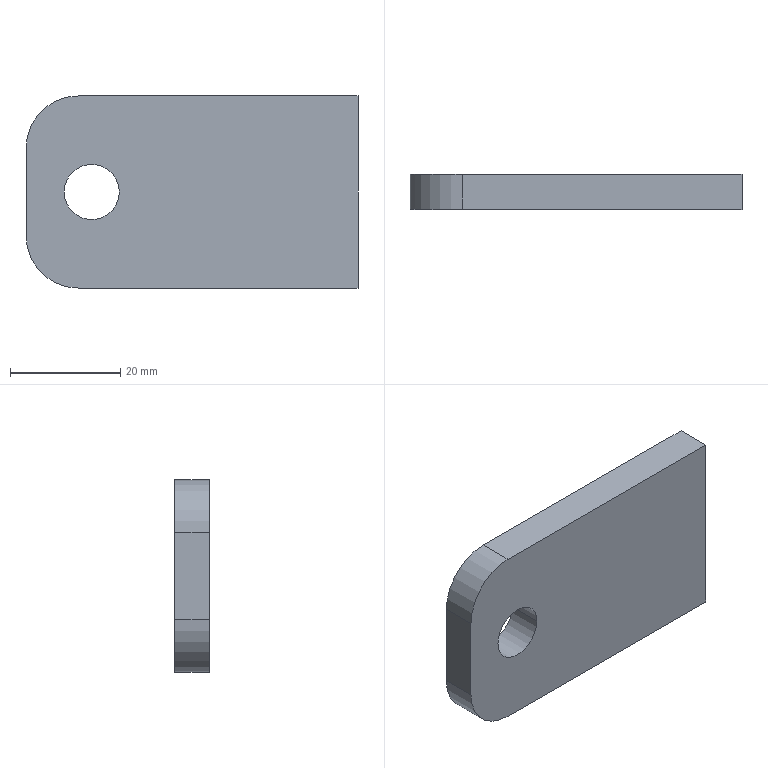Part | NX | features BREP 1 | 1 solid | 10 faces | box 60.325 x 6.35 x 34.925 mm | volume 12629 mm3 | plane 6 | cylinder 4 | commonest cylinder face diameters 10.033 x2 19.05 x2
STEP:
#1=CARTESIAN_POINT('',(0.,0.,-7.938));
#2=VERTEX_POINT('',#1);
#3=CARTESIAN_POINT('',(0.,0.,7.938));
#4=VERTEX_POINT('',#3);
#5=CARTESIAN_POINT('',(0.,0.,-7.938));
#6=DIRECTION('',(0.,0.,1.));
#7=VECTOR('',#6,1000.);
#8=LINE('',#5,#7);
#9=EDGE_CURVE('',#2,#4,#8,.T.);
#10=ORIENTED_EDGE('',*,*,#9,.T.);
#11=CARTESIAN_POINT('',(9.525,0.,17.462));
#12=VERTEX_POINT('',#11);
#13=CARTESIAN_POINT('',(9.525,0.,7.938));
#14=DIRECTION('',(0.,1.,0.));
#15=DIRECTION('',(-1.,0.,0.));
#16=AXIS2_PLACEMENT_3D('',#13,#14,#15);
#17=CIRCLE('',#16,9.525);
#18=EDGE_CURVE('',#4,#12,#17,.T.);
#19=ORIENTED_EDGE('',*,*,#18,.T.);
#20=CARTESIAN_POINT('',(60.325,0.,17.462));
#21=VERTEX_POINT('',#20);
#22=CARTESIAN_POINT('',(9.525,0.,17.462));
#23=DIRECTION('',(1.,0.,0.));
#24=VECTOR('',#23,1000.);
#25=LINE('',#22,#24);
#26=EDGE_CURVE('',#12,#21,#25,.T.);
#27=ORIENTED_EDGE('',*,*,#26,.T.);
#28=CARTESIAN_POINT('',(60.325,0.,-17.462));
#29=VERTEX_POINT('',#28);
#30=CARTESIAN_POINT('',(60.325,0.,17.462));
#31=DIRECTION('',(0.,0.,-1.));
#32=VECTOR('',#31,1000.);
#33=LINE('',#30,#32);
#34=EDGE_CURVE('',#21,#29,#33,.T.);
#35=ORIENTED_EDGE('',*,*,#34,.T.);
#36=CARTESIAN_POINT('',(9.525,0.,-17.462));
#37=VERTEX_POINT('',#36);
#38=CARTESIAN_POINT('',(60.325,0.,-17.462));
#39=DIRECTION('',(-1.,0.,0.));
#40=VECTOR('',#39,1000.);
#41=LINE('',#38,#40);
#42=EDGE_CURVE('',#29,#37,#41,.T.);
#43=ORIENTED_EDGE('',*,*,#42,.T.);
#44=CARTESIAN_POINT('',(9.525,0.,-7.938));
#45=DIRECTION('',(0.,1.,0.));
#46=DIRECTION('',(0.,0.,-1.));
#47=AXIS2_PLACEMENT_3D('',#44,#45,#46);
#48=CIRCLE('',#47,9.525);
#49=EDGE_CURVE('',#37,#2,#48,.T.);
#50=ORIENTED_EDGE('',*,*,#49,.T.);
#51=EDGE_LOOP('',(#10,#19,#27,#35,#43,#50));
#52=FACE_BOUND('',#51,.T.);
#53=CARTESIAN_POINT('',(16.954,0.,0.));
#54=VERTEX_POINT('',#53);
#55=CARTESIAN_POINT('',(6.921,0.,0.));
#56=VERTEX_POINT('',#55);
#57=CARTESIAN_POINT('',(11.938,0.,0.));
#58=DIRECTION('',(0.,1.,0.));
#59=DIRECTION('',(1.,0.,0.));
#60=AXIS2_PLACEMENT_3D('',#57,#58,#59);
#61=CIRCLE('',#60,5.016);
#62=EDGE_CURVE('',#54,#56,#61,.T.);
#63=ORIENTED_EDGE('',*,*,#62,.F.);
#64=CARTESIAN_POINT('',(11.938,0.,0.));
#65=DIRECTION('',(0.,1.,0.));
#66=DIRECTION('',(-1.,0.,0.));
#67=AXIS2_PLACEMENT_3D('',#64,#65,#66);
#68=CIRCLE('',#67,5.016);
#69=EDGE_CURVE('',#56,#54,#68,.T.);
#70=ORIENTED_EDGE('',*,*,#69,.F.);
#71=EDGE_LOOP('',(#63,#70));
#72=FACE_BOUND('',#71,.T.);
#73=CARTESIAN_POINT('',(0.,0.,0.));
#74=DIRECTION('',(0.,1.,0.));
#75=DIRECTION('',(1.,0.,0.));
#76=AXIS2_PLACEMENT_3D('',#73,#74,#75);
#77=PLANE('',#76);
#78=ADVANCED_FACE('',(#52,#72),#77,.T.);
#79=CARTESIAN_POINT('',(16.954,-6.35,0.));
#80=VERTEX_POINT('',#79);
#81=CARTESIAN_POINT('',(16.954,0.,0.));
#82=DIRECTION('',(0.,-1.,0.));
#83=VECTOR('',#82,1000.);
#84=LINE('',#81,#83);
#85=EDGE_CURVE('',#80,#54,#84,.F.);
#86=ORIENTED_EDGE('',*,*,#85,.F.);
#87=CARTESIAN_POINT('',(6.921,-6.35,0.));
#88=VERTEX_POINT('',#87);
#89=CARTESIAN_POINT('',(11.938,-6.35,0.));
#90=DIRECTION('',(0.,1.,0.));
#91=DIRECTION('',(-1.,0.,0.));
#92=AXIS2_PLACEMENT_3D('',#89,#90,#91);
#93=CIRCLE('',#92,5.016);
#94=EDGE_CURVE('',#88,#80,#93,.T.);
#95=ORIENTED_EDGE('',*,*,#94,.F.);
#96=CARTESIAN_POINT('',(6.921,0.,0.));
#97=DIRECTION('',(0.,-1.,0.));
#98=VECTOR('',#97,1000.);
#99=LINE('',#96,#98);
#100=EDGE_CURVE('',#88,#56,#99,.F.);
#101=ORIENTED_EDGE('',*,*,#100,.T.);
#102=ORIENTED_EDGE('',*,*,#69,.T.);
#103=EDGE_LOOP('',(#86,#95,#101,#102));
#104=FACE_BOUND('',#103,.T.);
#105=CARTESIAN_POINT('',(11.938,-3.175,0.));
#106=DIRECTION('',(0.,1.,0.));
#107=DIRECTION('',(-1.,0.,0.));
#108=AXIS2_PLACEMENT_3D('',#105,#106,#107);
#109=CYLINDRICAL_SURFACE('',#108,5.016);
#110=ADVANCED_FACE('',(#104),#109,.F.);
#111=ORIENTED_EDGE('',*,*,#100,.F.);
#112=CARTESIAN_POINT('',(11.938,-6.35,0.));
#113=DIRECTION('',(0.,1.,0.));
#114=DIRECTION('',(1.,0.,0.));
#115=AXIS2_PLACEMENT_3D('',#112,#113,#114);
#116=CIRCLE('',#115,5.016);
#117=EDGE_CURVE('',#80,#88,#116,.T.);
#118=ORIENTED_EDGE('',*,*,#117,.F.);
#119=ORIENTED_EDGE('',*,*,#85,.T.);
#120=ORIENTED_EDGE('',*,*,#62,.T.);
#121=EDGE_LOOP('',(#111,#118,#119,#120));
#122=FACE_BOUND('',#121,.T.);
#123=CARTESIAN_POINT('',(11.938,-3.175,0.));
#124=DIRECTION('',(0.,1.,0.));
#125=DIRECTION('',(1.,0.,0.));
#126=AXIS2_PLACEMENT_3D('',#123,#124,#125);
#127=CYLINDRICAL_SURFACE('',#126,5.016);
#128=ADVANCED_FACE('',(#122),#127,.F.);
#129=CARTESIAN_POINT('',(60.325,-6.35,-17.462));
#130=VERTEX_POINT('',#129);
#131=CARTESIAN_POINT('',(9.525,-6.35,-17.462));
#132=VERTEX_POINT('',#131);
#133=CARTESIAN_POINT('',(60.325,-6.35,-17.462));
#134=DIRECTION('',(-1.,0.,0.));
#135=VECTOR('',#134,1000.);
#136=LINE('',#133,#135);
#137=EDGE_CURVE('',#130,#132,#136,.T.);
#138=ORIENTED_EDGE('',*,*,#137,.F.);
#139=CARTESIAN_POINT('',(60.325,-6.35,17.462));
#140=VERTEX_POINT('',#139);
#141=CARTESIAN_POINT('',(60.325,-6.35,17.462));
#142=DIRECTION('',(0.,0.,-1.));
#143=VECTOR('',#142,1000.);
#144=LINE('',#141,#143);
#145=EDGE_CURVE('',#140,#130,#144,.T.);
#146=ORIENTED_EDGE('',*,*,#145,.F.);
#147=CARTESIAN_POINT('',(9.525,-6.35,17.462));
#148=VERTEX_POINT('',#147);
#149=CARTESIAN_POINT('',(9.525,-6.35,17.462));
#150=DIRECTION('',(1.,0.,0.));
#151=VECTOR('',#150,1000.);
#152=LINE('',#149,#151);
#153=EDGE_CURVE('',#148,#140,#152,.T.);
#154=ORIENTED_EDGE('',*,*,#153,.F.);
#155=CARTESIAN_POINT('',(0.,-6.35,7.938));
#156=VERTEX_POINT('',#155);
#157=CARTESIAN_POINT('',(9.525,-6.35,7.938));
#158=DIRECTION('',(0.,-1.,0.));
#159=DIRECTION('',(0.,0.,1.));
#160=AXIS2_PLACEMENT_3D('',#157,#158,#159);
#161=CIRCLE('',#160,9.525);
#162=EDGE_CURVE('',#148,#156,#161,.T.);
#163=ORIENTED_EDGE('',*,*,#162,.T.);
#164=CARTESIAN_POINT('',(0.,-6.35,-7.938));
#165=VERTEX_POINT('',#164);
#166=CARTESIAN_POINT('',(0.,-6.35,-7.938));
#167=DIRECTION('',(0.,0.,1.));
#168=VECTOR('',#167,1000.);
#169=LINE('',#166,#168);
#170=EDGE_CURVE('',#165,#156,#169,.T.);
#171=ORIENTED_EDGE('',*,*,#170,.F.);
#172=CARTESIAN_POINT('',(9.525,-6.35,-7.938));
#173=DIRECTION('',(0.,-1.,0.));
#174=DIRECTION('',(-1.,0.,0.));
#175=AXIS2_PLACEMENT_3D('',#172,#173,#174);
#176=CIRCLE('',#175,9.525);
#177=EDGE_CURVE('',#165,#132,#176,.T.);
#178=ORIENTED_EDGE('',*,*,#177,.T.);
#179=EDGE_LOOP('',(#138,#146,#154,#163,#171,#178));
#180=FACE_BOUND('',#179,.T.);
#181=ORIENTED_EDGE('',*,*,#117,.T.);
#182=ORIENTED_EDGE('',*,*,#94,.T.);
#183=EDGE_LOOP('',(#181,#182));
#184=FACE_BOUND('',#183,.T.);
#185=CARTESIAN_POINT('',(0.,-6.35,0.));
#186=DIRECTION('',(0.,1.,0.));
#187=DIRECTION('',(1.,0.,0.));
#188=AXIS2_PLACEMENT_3D('',#185,#186,#187);
#189=PLANE('',#188);
#190=ADVANCED_FACE('',(#180,#184),#189,.F.);
#191=ORIENTED_EDGE('',*,*,#177,.F.);
#192=CARTESIAN_POINT('',(0.,-6.35,-7.938));
#193=DIRECTION('',(0.,1.,0.));
#194=VECTOR('',#193,1000.);
#195=LINE('',#192,#194);
#196=EDGE_CURVE('',#165,#2,#195,.T.);
#197=ORIENTED_EDGE('',*,*,#196,.T.);
#198=ORIENTED_EDGE('',*,*,#49,.F.);
#199=CARTESIAN_POINT('',(9.525,-6.35,-17.462));
#200=DIRECTION('',(0.,1.,0.));
#201=VECTOR('',#200,1000.);
#202=LINE('',#199,#201);
#203=EDGE_CURVE('',#132,#37,#202,.T.);
#204=ORIENTED_EDGE('',*,*,#203,.F.);
#205=EDGE_LOOP('',(#191,#197,#198,#204));
#206=FACE_BOUND('',#205,.T.);
#207=CARTESIAN_POINT('',(9.525,-6.45,-7.938));
#208=DIRECTION('',(0.,1.,0.));
#209=DIRECTION('',(0.,0.,-1.));
#210=AXIS2_PLACEMENT_3D('',#207,#208,#209);
#211=CYLINDRICAL_SURFACE('',#210,9.525);
#212=ADVANCED_FACE('',(#206),#211,.T.);
#213=ORIENTED_EDGE('',*,*,#42,.F.);
#214=CARTESIAN_POINT('',(60.325,0.,-17.462));
#215=DIRECTION('',(0.,-1.,0.));
#216=VECTOR('',#215,1000.);
#217=LINE('',#214,#216);
#218=EDGE_CURVE('',#29,#130,#217,.T.);
#219=ORIENTED_EDGE('',*,*,#218,.T.);
#220=ORIENTED_EDGE('',*,*,#137,.T.);
#221=ORIENTED_EDGE('',*,*,#203,.T.);
#222=EDGE_LOOP('',(#213,#219,#220,#221));
#223=FACE_BOUND('',#222,.T.);
#224=CARTESIAN_POINT('',(30.163,-3.175,-17.462));
#225=DIRECTION('',(0.,0.,-1.));
#226=DIRECTION('',(0.,-1.,0.));
#227=AXIS2_PLACEMENT_3D('',#224,#225,#226);
#228=PLANE('',#227);
#229=ADVANCED_FACE('',(#223),#228,.T.);
#230=CARTESIAN_POINT('',(60.325,0.,17.462));
#231=DIRECTION('',(0.,-1.,0.));
#232=VECTOR('',#231,1000.);
#233=LINE('',#230,#232);
#234=EDGE_CURVE('',#21,#140,#233,.T.);
#235=ORIENTED_EDGE('',*,*,#234,.T.);
#236=ORIENTED_EDGE('',*,*,#145,.T.);
#237=ORIENTED_EDGE('',*,*,#218,.F.);
#238=ORIENTED_EDGE('',*,*,#34,.F.);
#239=EDGE_LOOP('',(#235,#236,#237,#238));
#240=FACE_BOUND('',#239,.T.);
#241=CARTESIAN_POINT('',(60.325,-3.175,0.));
#242=DIRECTION('',(1.,0.,0.));
#243=DIRECTION('',(0.,1.,0.));
#244=AXIS2_PLACEMENT_3D('',#241,#242,#243);
#245=PLANE('',#244);
#246=ADVANCED_FACE('',(#240),#245,.T.);
#247=ORIENTED_EDGE('',*,*,#153,.T.);
#248=ORIENTED_EDGE('',*,*,#234,.F.);
#249=ORIENTED_EDGE('',*,*,#26,.F.);
#250=CARTESIAN_POINT('',(9.525,-6.35,17.462));
#251=DIRECTION('',(0.,1.,0.));
#252=VECTOR('',#251,1000.);
#253=LINE('',#250,#252);
#254=EDGE_CURVE('',#148,#12,#253,.T.);
#255=ORIENTED_EDGE('',*,*,#254,.F.);
#256=EDGE_LOOP('',(#247,#248,#249,#255));
#257=FACE_BOUND('',#256,.T.);
#258=CARTESIAN_POINT('',(30.163,-3.175,17.462));
#259=DIRECTION('',(0.,0.,1.));
#260=DIRECTION('',(1.,0.,0.));
#261=AXIS2_PLACEMENT_3D('',#258,#259,#260);
#262=PLANE('',#261);
#263=ADVANCED_FACE('',(#257),#262,.T.);
#264=ORIENTED_EDGE('',*,*,#162,.F.);
#265=ORIENTED_EDGE('',*,*,#254,.T.);
#266=ORIENTED_EDGE('',*,*,#18,.F.);
#267=CARTESIAN_POINT('',(0.,-6.35,7.938));
#268=DIRECTION('',(0.,1.,0.));
#269=VECTOR('',#268,1000.);
#270=LINE('',#267,#269);
#271=EDGE_CURVE('',#156,#4,#270,.T.);
#272=ORIENTED_EDGE('',*,*,#271,.F.);
#273=EDGE_LOOP('',(#264,#265,#266,#272));
#274=FACE_BOUND('',#273,.T.);
#275=CARTESIAN_POINT('',(9.525,-6.45,7.938));
#276=DIRECTION('',(0.,1.,0.));
#277=DIRECTION('',(-1.,0.,0.));
#278=AXIS2_PLACEMENT_3D('',#275,#276,#277);
#279=CYLINDRICAL_SURFACE('',#278,9.525);
#280=ADVANCED_FACE('',(#274),#279,.T.);
#281=ORIENTED_EDGE('',*,*,#170,.T.);
#282=ORIENTED_EDGE('',*,*,#271,.T.);
#283=ORIENTED_EDGE('',*,*,#9,.F.);
#284=ORIENTED_EDGE('',*,*,#196,.F.);
#285=EDGE_LOOP('',(#281,#282,#283,#284));
#286=FACE_BOUND('',#285,.T.);
#287=CARTESIAN_POINT('',(0.,-3.175,0.));
#288=DIRECTION('',(-1.,0.,0.));
#289=DIRECTION('',(0.,0.,1.));
#290=AXIS2_PLACEMENT_3D('',#287,#288,#289);
#291=PLANE('',#290);
#292=ADVANCED_FACE('',(#286),#291,.T.);
#293=CLOSED_SHELL('',(#78,#110,#128,#190,#212,#229,#246,#263,#280,#292));
#294=MANIFOLD_SOLID_BREP('',#293);
#295=(LENGTH_UNIT()NAMED_UNIT(*)SI_UNIT(.MILLI.,.METRE.));
#296=UNCERTAINTY_MEASURE_WITH_UNIT(LENGTH_MEASURE(0.00001),#295,'','');
#297=(NAMED_UNIT(*)PLANE_ANGLE_UNIT()SI_UNIT($,.RADIAN.));
#298=(NAMED_UNIT(*)SI_UNIT($,.STERADIAN.)SOLID_ANGLE_UNIT());
#299=(GEOMETRIC_REPRESENTATION_CONTEXT(3)GLOBAL_UNCERTAINTY_ASSIGNED_CONTEXT((#296))GLOBAL_UNIT_ASSIGNED_CONTEXT((#295,#297,#298))REPRESENTATION_CONTEXT('',''));
#300=ADVANCED_BREP_SHAPE_REPRESENTATION('',(#294),#299);